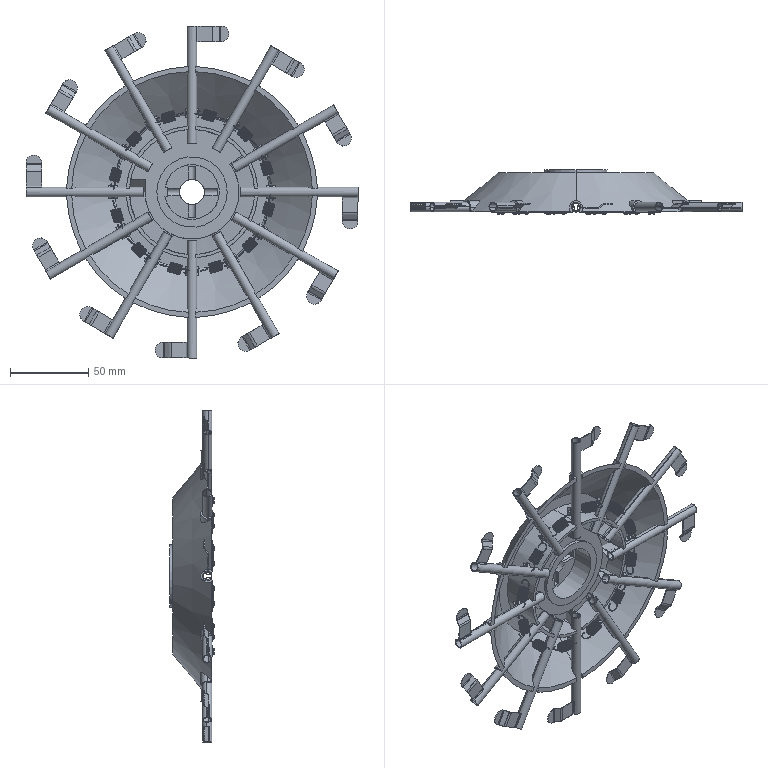Part | SolidWorks | features ReferencePattern 22, LocalCirPattern 2 | 26 solids | 951 faces | box 212 x 28.613 x 212 mm | volume 113831 mm3 | plane 421 | cylinder 356 | spline 170 | cone 4 | commonest cylinder face diameters 6 x96 5 x76 4 x60 1.5 x48 1 x12 2 x12